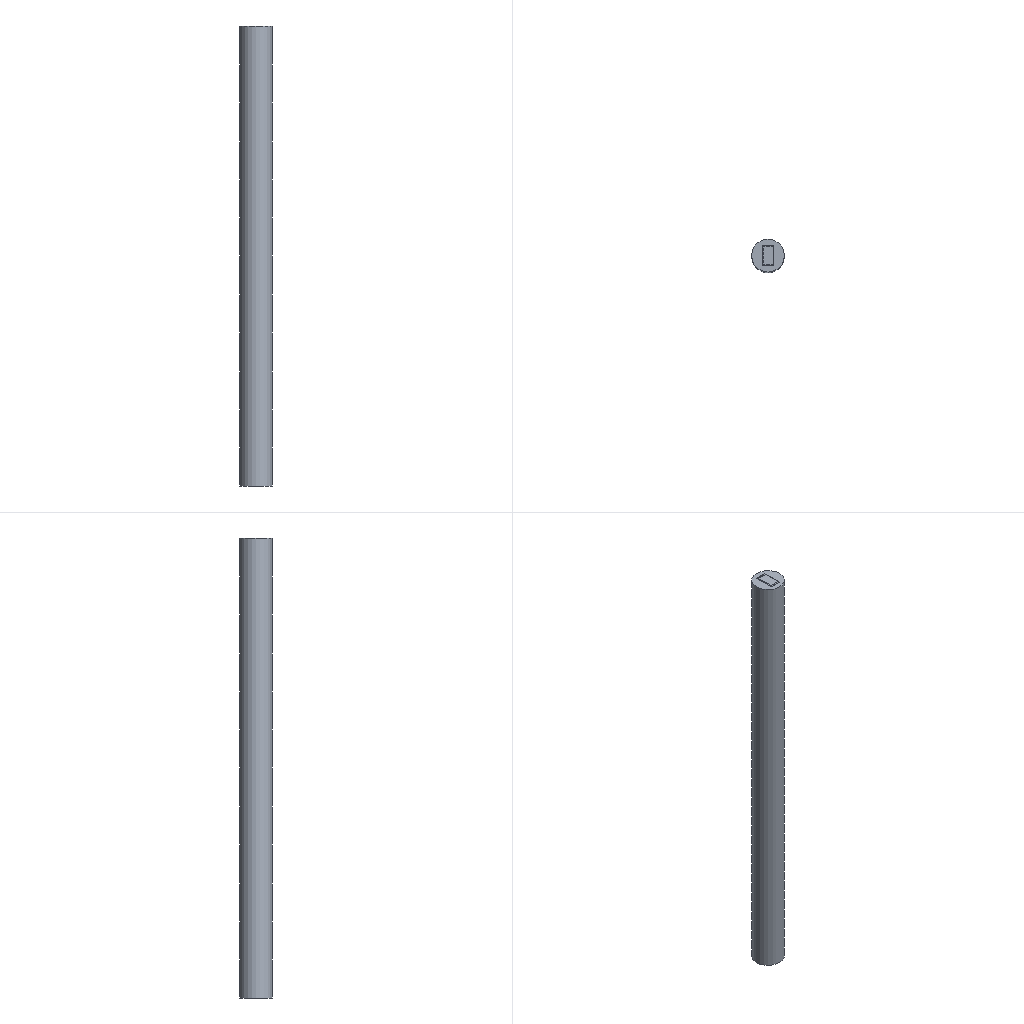Simulation study | abaqus
Set-up summary:
category,name,step,type,value,unit,region
solver,abaqus,,Abaqus/CAE 2024
units,mm-N-s-tonne (MPa),,inferred,E=206000 density=7.85e-09
analysis,Step-1,,dynamic explicit,nlgeom=True; time_period=0.02
mesh,nodes,,,88958
mesh,elements,,,66642
element_type,C3D8R,,,63378
element_type,S4R,,,2688
element_type,R3D4,,,384
element_type,T3D2,,,175
element_type,R3D3,,,16
element_type,MASS,,,1
material,CAOGANG,,E,206000
material,CAOGANG,,nu,0.3
material,CAOGANG,,density,7.85e-09
material,CAOGANG,,yield,235.322
material,CAOGANG,,behaviors,plastic; damage initiation; damage evolution
material,GFRP,,E,126000
material,GFRP,,nu,0.3
material,GFRP,,density,2e-09
material,GFRP,,behaviors,damage initiation; elastic engineering constants
material,HUNNINGTU,,E,36000
material,HUNNINGTU,,nu,0.25
material,HUNNINGTU,,density,2.5e-09
material,HUNNINGTU,,behaviors,plastic; concrete damaged plasticity; concrete compression hardening; concrete tension stiffening
material,gangjiaoxian,,E,195000
material,gangjiaoxian,,nu,0.3
material,gangjiaoxian,,density,7.85e-09
material,gangjiaoxian,,cte,1.2e-05
material,gangjiaoxian,,behaviors,expansion
section,CAOGANG,,solid section,,,_PickedSet15
section,,,shell section,0.1,,GFRP-1
section,HUNNINGTU,,solid section,,,_PickedSet3
section,HUNNINGTU,,solid section,,,_PickedSet2
section,gangjiaoxian,,solid section,,,_PickedSet2
load,Predefined,initial,initial condition temperature
load,qiu150,initial,initial condition velocity
load,Predefined,Step-1,temperature,-325,,Set-16
bc,gudingduan,initial,encastre,[dofs=ENCASTRE],,_PickedSet51
bc,qiu150,initial,fixed,"[dofs=rx,ry,rz,x,z n=5]",,_PickedSet89
bc,shuxiang,initial,fixed,"[dofs=rx,ry,rz,x,z n=5]",,_PickedSet52
contact,tu1-tu2,initial,tie,,,_PickedSurf47 / _PickedSurf46
contact,caonei-tu2,Step-1,contact pair,interaction=caonei-tu2; friction=0.6; behavior=hard,,_PickedSurf44 / _PickedSurf45
contact,caowai-tu1,Step-1,contact pair,interaction=caowai-tu1; friction=0.6; behavior=hard,,_PickedSurf42 / _PickedSurf43
contact,gfrp-hunningtu1,Step-1,contact pair,interaction=gfrp-hunningtu1; friction=0.6; behavior=hard,,_PickedSurf40 / _PickedSurf41
contact,qiu150-gfrp,Step-1,contact pair,interaction=qiu150-gfrp; friction=0; behavior=hard,,_PickedSurf67 / _PickedSurf68
constraint,embedded element,,,1
constraint,coupling,,,2
constraint,rigid body,,,1
Abaqus input file, long lists of numbers shortened:
*Heading
** Job name: deck Model name: CFFT-SP3-150-135-Copy
** Generated by: Abaqus/CAE 2024
*Preprint, echo=NO, model=NO, history=NO, contact=NO
**
** PARTS
**
*Part, name=CAOGANG
*Node
      1,          65.,          92.,           0.
      2,          65.,          92.,        1400.
** (22462 more lines like these left out)
*Element, type=C3D8R
   1,     8,  1091,  7807,  1453,     1,    21,  3619,   742
   2,  1091,  1090,  7808,  7807,    21,    22,  3620,  3619
** (10848 more lines like these left out)
*Nset, nset=Set-1, generate
     1,  22464,      1
*Elset, elset=Set-1, generate
     1,  10850,      1
*Nset, nset=_PickedSet15, internal, generate
     1,  22464,      1
*Elset, elset=_PickedSet15, internal, generate
     1,  10850,      1
** Section: CAOGANG
*Solid Section, elset=_PickedSet15, material=CAOGANG
,
*End Part
**
*Part, name=GFRP
*Node
      1,         -50.,           0.,        1400.
      2,         -50.,           0.,        1250.
** (2710 more lines like these left out)
*Element, type=S4R
 1,    1,   81, 1065,  108
 2,   81,   82, 1066, 1065
** (2686 more lines like these left out)
*Nset, nset=_PickedSet6, internal
    1,    4,   22,   25,   43,   46,   62,   65,  106,  107,  108,  345,  346,  347,  582,  799
  993, 1001, 1002, 1003, 1009, 1016, 1017, 1018
*Elset, elset=_PickedSet6, internal
    1,   13,   25,   37,  449,  461,  473,  485,  897,  909, 1121, 1133, 1356, 1368, 1428, 1440
 1452, 1464, 1500, 1512, 1572, 1584, 1596, 1608
*Elset, elset=__PickedSurf5_SPOS, internal, generate
    1,  2688,     1
*Surface, type=ELEMENT, name=_PickedSurf5, internal
__PickedSurf5_SPOS, SPOS
*Distribution, name=Ori-1-DiscOrient, location=ELEMENT, Table=Ori-1-DiscOrient_Table
** Description: Distribution generated from Discrete Orientation
,           1.,           0.,           0.,           0.,           1.,           0.
1, -0.1326, 0.9912,           0.,           0.,           0.,          -1.
2, -0.1326, 0.9912,           0.,           0.,           0.,          -1.
3, -0.1326, 0.9912,           0.,           0.,           0.,          -1.
4, -0.1326, 0.9912,           0.,           0.,           0.,          -1.
5, -0.1326, 0.9912,           0.,           0.,           0.,          -1.
6, -0.1326, 0.9912,           0.,           0.,           0.,          -1.
7, -0.1326, 0.9912,           0.,           0.,           0.,          -1.
8, -0.1326, 0.9912,           0.,           0.,           0.,          -1.
9, -0.1326, 0.9912,           0.,           0.,           0.,          -1.
10, -0.1326, 0.9912,           0.,           0.,           0.,          -1.
11, -0.1326, 0.9912,           0.,           0.,           0.,          -1.
12, -0.1326, 0.9912,           0.,           0.,           0.,          -1.
13, -0.3884, 0.9215,           0.,           0.,           0.,          -1.
14, -0.3884, 0.9215,           0.,           0.,           0.,          -1.
15, -0.3884, 0.9215,           0.,           0.,           0.,          -1.
16, -0.3884, 0.9215,           0.,           0.,           0.,          -1.
17, -0.3884, 0.9215,           0.,           0.,           0.,          -1.
18, -0.3884, 0.9215,           0.,           0.,           0.,          -1.
19, -0.3884, 0.9215,           0.,           0.,           0.,          -1.
20, -0.3884, 0.9215,           0.,           0.,           0.,          -1.
21, -0.3884, 0.9215,           0.,           0.,           0.,          -1.
22, -0.3884, 0.9215,           0.,           0.,           0.,          -1.
23, -0.3884, 0.9215,           0.,           0.,           0.,          -1.
24, -0.3884, 0.9215,           0.,           0.,           0.,          -1.
25, -0.6169, 0.787,           0.,           0.,           0.,          -1.
26, -0.6169, 0.787,           0.,           0.,           0.,          -1.
27, -0.6169, 0.787,           0.,           0.,           0.,          -1.
28, -0.6169, 0.787,           0.,           0.,           0.,          -1.
29, -0.6169, 0.787,           0.,           0.,           0.,          -1.
30, -0.6169, 0.787,           0.,           0.,           0.,          -1.
31, -0.6169, 0.787,           0.,           0.,           0.,          -1.
32, -0.6169, 0.787,           0.,           0.,           0.,          -1.
33, -0.6169, 0.787,           0.,           0.,           0.,          -1.
34, -0.6169, 0.787,           0.,           0.,           0.,          -1.
35, -0.6169, 0.787,           0.,           0.,           0.,          -1.
36, -0.6169, 0.787,           0.,           0.,           0.,          -1.
37, -0.8021, 0.5972,           0.,           0.,           0.,          -1.
38, -0.8021, 0.5972,           0.,           0.,           0.,          -1.
39, -0.8021, 0.5972,           0.,           0.,           0.,          -1.
** (2649 more lines like these left out)
*Orientation, name=Ori-1, system=RECTANGULAR
Ori-1-DiscOrient
3, 0.
** Region: (GFRP-1: Generated From Layup)
*Elset, elset=GFRP-1, generate
    1,  2688,     1
** Section: GFRP-1
*Shell Section, elset=GFRP-1, composite, orientation=Ori-1, offset=SNEG, layup=GFRP
0.1, 3, GFRP, 80., 层-1
0.1, 3, GFRP, -80., 层-2
0.1, 3, GFRP, 80., 层-3
*End Part
**
*Part, name=HUNNINGTU1
*Node
      1,        -17.5,           0.,        1400.
      2,         -50.,           0.,        1400.
** (18982 more lines like these left out)
*Element, type=C3D8R
   1,   286,  2649, 10105,  1983,     1,    33,  1953,    48
   2,  2649,  2650, 10106, 10105,    33,    34,  1954,  1953
** (16126 more lines like these left out)
*Nset, nset=_PickedSet3, internal, generate
     1,  18984,      1
*Elset, elset=_PickedSet3, internal, generate
     1,  16128,      1
** Section: HUNNINGTU
*Solid Section, elset=_PickedSet3, material=HUNNINGTU
,
*End Part
**
*Part, name=HUNNINGTU2
*Node
      1,         100.,          97.,        1400.
      2,       96.125,          97.,        1400.
** (44224 more lines like these left out)
*Element, type=C3D8R
    1,  3160,  3161,  3170,  3169,     1,     2,    11,    10
    2,  3161,  3162,  3171,  3170,     2,     3,    12,    11
** (36398 more lines like these left out)
*Nset, nset=_PickedSet2, internal, generate
     1,  44226,      1
*Elset, elset=_PickedSet2, internal, generate
     1,  36400,      1
** Section: HUNNINGTU
*Solid Section, elset=_PickedSet2, material=HUNNINGTU
,
*End Part
**
*Part, name=QIU100
*Node
      1,          50.,           0.,           0.
      2,           0.,           0.,          50.
** (392 more lines like these left out)
*Element, type=R3D3
1, 108, 107, 122
2, 126, 113, 109
** (14 more lines like these left out)
*Element, type=R3D4
 3,   7,  93,  27,   1
 4, 114,  93,  92, 115
** (382 more lines like these left out)
*End Part
**
*Part, name=gangjiaoxian
*Node
      1,       -1075.,           0.,           0.
      2,       -1067.,           0.,           0.
** (174 more lines like these left out)
*Element, type=T3D2
  1,   1,   2
  2,   2,   3
** (173 more lines like these left out)
*Nset, nset=_PickedSet2, internal, generate
   1,  176,    1
*Elset, elset=_PickedSet2, internal, generate
   1,  175,    1
** Section: gangjiaoxian
*Solid Section, elset=_PickedSet2, material=gangjiaoxian
140.,
*End Part
**
**
** ASSEMBLY
**
*Assembly, name=Assembly
**
*Instance, name=GFRP-1, part=GFRP
*End Instance
**
*Instance, name=HUNNINGTU1-1, part=HUNNINGTU1
*End Instance
**
*Instance, name=CAOGANG-1, part=CAOGANG
       -82.5,       -118.5,           0.
*End Instance
**
*Instance, name=HUNNINGTU2-1, part=HUNNINGTU2
       -82.5,       -123.5,           0.
*End Instance
**
*Instance, name=QIU100-1, part=QIU100
          0.,         176.,        1250.
*End Instance
**
*Instance, name=gangjiaoxian-1, part=gangjiaoxian
7.95145259115256e-14,           0., 325.
7.95145259115256e-14,           0., 325., 7.95145259115256e-14, 1., 325., 90.
*End Instance
**
*Node
      1,           0.,           0.,           0.
*Node
      2,           0.,         226.,        1250.
*Nset, nset=Set-16, instance=gangjiaoxian-1, generate
   1,  176,    1
*Elset, elset=Set-16, instance=gangjiaoxian-1, generate
   1,  175,    1
*Nset, nset=jiasudu, instance=HUNNINGTU1-1
 1373, 1405, 1433
*Nset, nset=weiyi, instance=HUNNINGTU1-1
   21, 1369, 1393, 1417, 1441
*Nset, nset=yingbian, instance=HUNNINGTU1-1
   21, 1349, 1365, 1377, 1401, 1413, 1437
*Nset, nset=_PickedSet51, internal, instance=HUNNINGTU1-1
    5,    6,    7,    8,   13,   14,   15,   16,   21,   22,   23,   24,   27,   28,   31,   32
   49,   50,   51,   52,   53,   54,   55,   56,   57,   58,   59,   60,   61,   62,   63,   64
** (9 more lines like these left out)
*Nset, nset=_PickedSet51, internal, instance=CAOGANG-1
    1,    4,    7,    8,   11,   12,   14,   17,   18,   19,  731,  732,  733,  734,  735,  736
  737,  738,  739,  740,  741,  742, 1453, 1454, 1455, 1456, 1457, 1458, 1459, 1460, 1461, 1462
** (2 more lines like these left out)
*Nset, nset=_PickedSet51, internal, instance=HUNNINGTU2-1
  3151,  3152,  3153,  3154,  3155,  3156,  3157,  3158,  3159,  6310,  6311,  6312,  6313,  6314,  6315,  6316
  6317,  6318,  9469,  9470,  9471,  9472,  9473,  9474,  9475,  9476,  9477, 12628, 12629, 12630, 12631, 12632
** (6 more lines like these left out)
*Elset, elset=_PickedSet51, internal, instance=HUNNINGTU1-1
  2665,  2666,  2667,  2668,  2669,  2670,  2671,  2672,  2673,  2674,  2675,  2676,  2677,  2678,  2679,  2680
  2681,  2682,  2683,  2684,  2685,  2686,  2687,  2688,  5353,  5354,  5355,  5356,  5357,  5358,  5359,  5360
** (7 more lines like these left out)
*Elset, elset=_PickedSet51, internal, instance=CAOGANG-1
     1,   351,   701,  1051,  1401,  1751,  2101,  2451,  2801,  3151,  3501,  3851,  4201,  4900,  5250,  5600
  5950,  6300,  6650,  7000,  7350,  7700,  8050,  8400,  8750,  9100,  9450,  9800, 10150, 10500, 10850
*Elset, elset=_PickedSet51, internal, instance=HUNNINGTU2-1
  2793,  2794,  2795,  2796,  2797,  2798,  2799,  2800,  5593,  5594,  5595,  5596,  5597,  5598,  5599,  5600
  8393,  8394,  8395,  8396,  8397,  8398,  8399,  8400, 11193, 11194, 11195, 11196, 11197, 11198, 11199, 11200
** (5 more lines like these left out)
*Nset, nset=_PickedSet52, internal, instance=HUNNINGTU1-1
   2,   5,  10,  13, 398, 399, 400, 401, 402, 403, 404, 405, 406, 407, 408, 409
 410, 411, 412, 413, 414, 415, 416, 417, 418, 419, 420, 421, 422, 423, 424, 425
** (13 more lines like these left out)
*Elset, elset=_PickedSet52, internal, instance=HUNNINGTU1-1
     6,    30,    54,    78,   102,   126,   150,   174,   198,   222,   246,   270,   294,   318,   342,   366
   390,   414,   438,   462,   486,   510,   534,   558,   582,   606,   630,   654,   678,   702,   726,   750
** (26 more lines like these left out)
*Nset, nset=_PickedSet62, internal
 1,
*Nset, nset=_PickedSet63, internal, instance=HUNNINGTU1-1
    5,    6,   13,   14,   21,   22,   28,   32,   54,   55,   56,  530,  531,  532, 1002, 1466
 1708, 1709, 1710, 1942, 1943, 1944, 1947, 1952
*Elset, elset=_PickedSet63, internal, instance=HUNNINGTU1-1
  2670,  2676,  2682,  2688,  5358,  5364,  5370,  5376,  6714,  6720,  8053,  8059, 10729, 10735, 10741, 10747
 13417, 13423, 13429, 13435, 14778, 14784, 16117, 16123
*Nset, nset=_PickedSet64, internal
 1,
*Nset, nset=_PickedSet71, internal, instance=QIU100-1, generate
   1,  394,    1
*Elset, elset=_PickedSet71, internal, instance=QIU100-1, generate
   1,  400,    1
*Nset, nset=_PickedSet84, internal, instance=gangjiaoxian-1, generate
   1,  176,    1
*Elset, elset=_PickedSet84, internal, instance=gangjiaoxian-1, generate
   1,  175,    1
*Nset, nset=_PickedSet87, internal
 2,
*Nset, nset=_PickedSet88, internal
 2,
*Nset, nset=_PickedSet89, internal
 2,
*Elset, elset=__PickedSurf40_SNEG, internal, instance=GFRP-1, generate
    1,  2688,     1
*Surface, type=ELEMENT, name=_PickedSurf40, internal
__PickedSurf40_SNEG, SNEG
*Elset, elset=__PickedSurf41_S4, internal, instance=HUNNINGTU1-1
     6,    12,    18,    24,    30,    36,    42,    48,    54,    60,    66,    72,    78,    84,    90,    96
   102,   108,   114,   120,   126,   132,   138,   144,   150,   156,   162,   168,   174,   180,   186,   192
** (82 more lines like these left out)
*Elset, elset=__PickedSurf41_S6, internal, instance=HUNNINGTU1-1
  6721,  6727,  6733,  6739,  6745,  6751,  6757,  6763,  6769,  6775,  6781,  6787,  6793,  6799,  6805,  6811
  6817,  6823,  6829,  6835,  6841,  6847,  6853,  6859,  6865,  6871,  6877,  6883,  6889,  6895,  6901,  6907
** (82 more lines like these left out)
*Surface, type=ELEMENT, name=_PickedSurf41, internal
__PickedSurf41_S4, S4
__PickedSurf41_S6, S6
*Elset, elset=__PickedSurf42_S2, internal, instance=CAOGANG-1
    1,    2,    3,    4,    5,    6,    7,    8,    9,   10,   11,   12,   13,   14,   15,   16
   17,   18,   19,   20,   21,   22,   23,   24,   25,   26,   27,   28,   29,   30,   31,   32
** (327 more lines like these left out)
*Elset, elset=__PickedSurf42_S1, internal, instance=CAOGANG-1
  7351,  7352,  7353,  7354,  7355,  7356,  7357,  7358,  7359,  7360,  7361,  7362,  7363,  7364,  7365,  7366
  7367,  7368,  7369,  7370,  7371,  7372,  7373,  7374,  7375,  7376,  7377,  7378,  7379,  7380,  7381,  7382
** (42 more lines like these left out)
*Elset, elset=__PickedSurf42_S6, internal, instance=CAOGANG-1, generate
  7701,  10850,      1
*Elset, elset=__PickedSurf42_S4, internal, instance=CAOGANG-1, generate
 4551,  7700,     1
*Surface, type=ELEMENT, name=_PickedSurf42, internal
__PickedSurf42_S2, S2
__PickedSurf42_S1, S1
__PickedSurf42_S6, S6
__PickedSurf42_S4, S4
*Elset, elset=__PickedSurf43_S4, internal, instance=HUNNINGTU1-1
  6726,  6732,  6738,  6744,  6750,  6756,  6762,  6768,  6774,  6780,  6786,  6792,  6798,  6804,  6810,  6816
  6822,  6828,  6834,  6840,  6846,  6852,  6858,  6864,  6870,  6876,  6882,  6888,  6894,  6900,  6906,  6912
** (82 more lines like these left out)
*Elset, elset=__PickedSurf43_S6, internal, instance=HUNNINGTU1-1
     1,     7,    13,    19,    25,    31,    37,    43,    49,    55,    61,    67,    73,    79,    85,    91
    97,   103,   109,   115,   121,   127,   133,   139,   145,   151,   157,   163,   169,   175,   181,   187
** (82 more lines like these left out)
*Surface, type=ELEMENT, name=_PickedSurf43, internal
__PickedSurf43_S4, S4
__PickedSurf43_S6, S6
*Elset, elset=__PickedSurf44_S4, internal, instance=CAOGANG-1, generate
  7701,  10500,      1
*Elset, elset=__PickedSurf44_S1, internal, instance=CAOGANG-1, generate
    1,  4550,     1
*Elset, elset=__PickedSurf44_S6, internal, instance=CAOGANG-1, generate
 4551,  7350,     1
*Surface, type=ELEMENT, name=_PickedSurf44, internal
__PickedSurf44_S4, S4
__PickedSurf44_S1, S1
__PickedSurf44_S6, S6
*Elset, elset=__PickedSurf45_S1, internal, instance=HUNNINGTU2-1, generate
 33601,  36400,      1
*Elset, elset=__PickedSurf45_S2, internal, instance=HUNNINGTU2-1, generate
    1,  2800,     1
*Elset, elset=__PickedSurf45_S4, internal, instance=HUNNINGTU2-1, generate
     8,  36400,      8
*Surface, type=ELEMENT, name=_PickedSurf45, internal
__PickedSurf45_S1, S1
__PickedSurf45_S2, S2
__PickedSurf45_S4, S4
*Elset, elset=__PickedSurf46_S4, internal, instance=HUNNINGTU1-1, generate
  8070,  10752,      6
*Elset, elset=__PickedSurf46_S6, internal, instance=HUNNINGTU1-1, generate
 2689,  5371,     6
*Surface, type=ELEMENT, name=_PickedSurf46, internal
__PickedSurf46_S4, S4
__PickedSurf46_S6, S6
*Elset, elset=__PickedSurf47_S6, internal, instance=HUNNINGTU2-1, generate
     1,  36393,      8
*Surface, type=ELEMENT, name=_PickedSurf47, internal
__PickedSurf47_S6, S6
*Elset, elset=__PickedSurf61_S1, internal, instance=HUNNINGTU1-1
  2665,  2666,  2667,  2668,  2669,  2670,  2671,  2672,  2673,  2674,  2675,  2676,  2677,  2678,  2679,  2680
  2681,  2682,  2683,  2684,  2685,  2686,  2687,  2688,  5353,  5354,  5355,  5356,  5357,  5358,  5359,  5360
** (7 more lines like these left out)
*Elset, elset=__PickedSurf61_S5, internal, instance=CAOGANG-1, generate
  4900,  10850,    350
*Elset, elset=__PickedSurf61_S5, internal, instance=HUNNINGTU2-1
  2793,  2794,  2795,  2796,  2797,  2798,  2799,  2800,  5593,  5594,  5595,  5596,  5597,  5598,  5599,  5600
  8393,  8394,  8395,  8396,  8397,  8398,  8399,  8400, 11193, 11194, 11195, 11196, 11197, 11198, 11199, 11200
** (5 more lines like these left out)
*Elset, elset=__PickedSurf61_S6, internal, instance=CAOGANG-1, generate
    1,  4201,   350
*Surface, type=ELEMENT, name=_PickedSurf61, internal
__PickedSurf61_S1, S1
__PickedSurf61_S5, S5
__PickedSurf61_S6, S6
*Elset, elset=__PickedSurf67_SPOS, internal, instance=QIU100-1
   1,   2,   3,   4,   5,   6,   7,   8,   9,  10,  11,  12,  13,  14,  15,  16
  17,  18,  19,  20,  21,  22,  23,  24,  25,  26,  27,  28,  29,  30,  31,  32
** (11 more lines like these left out)
*Surface, type=ELEMENT, name=_PickedSurf67, internal
__PickedSurf67_SPOS, SPOS
*Elset, elset=__PickedSurf68_SPOS, internal, instance=GFRP-1
    1,    2,    3,    4,    5,    6,    7,    8,    9,   10,   11,   12,   13,   14,   15,   16
   17,   18,   19,   20,   21,   22,   23,   24,   25,   26,   27,   28,   29,   30,   31,   32
** (34 more lines like these left out)
*Surface, type=ELEMENT, name=_PickedSurf68, internal
__PickedSurf68_SPOS, SPOS
*Surface, type=NODE, name=_PickedSet63_CNS_, internal
_PickedSet63, 1.
** Constraint: gangjioaxian-hun2
*Embedded Element
_PickedSet84
** Constraint: guding-gfrp
*Coupling, constraint name=guding-gfrp, ref node=_PickedSet64, surface=_PickedSet63_CNS_
*Kinematic
** Constraint: gudingduan
*Coupling, constraint name=gudingduan, ref node=_PickedSet62, surface=_PickedSurf61
*Kinematic
** Constraint: qiu150
*Rigid Body, ref node=_PickedSet87, elset=_PickedSet71
** Constraint: tu1-tu2
*Tie, name=tu1-tu2, adjust=yes
_PickedSurf47, _PickedSurf46
*Element, type=MASS, elset=_PickedSet86_qiu150_
1, 2
*Mass, elset=_PickedSet86_qiu150_
0.0139,
*End Assembly
*Distribution Table, name=Ori-1-DiscOrient_Table
coord3D, coord3D
*Amplitude, name=Amp-1
             0.,              0.,            0.01,              1.
**
** MATERIALS
**
*Material, name=CAOGANG
*Damage Initiation, criterion=DUCTILE
 0.44,  1.29, 4.375
*Damage Evolution, type=DISPLACEMENT
 8.8,
*Density
 7.85e-09,
*Elastic
206000., 0.3
*Plastic
 235.322,         0.
 235.611, 0.001454
 235.901, 0.002681
  236.19, 0.003906
  236.48, 0.005129
 236.769, 0.006352
 237.059, 0.007572
 237.348, 0.008791
 237.638,  0.01001
 237.927,  0.01123
 238.217,  0.01244
 255.579,  0.02444
 273.288,  0.03629
 291.345,  0.048
  309.75,  0.05956
 328.501,  0.071
 347.601,  0.0823
 367.047,  0.09347
 386.841,   0.1045
 406.983,   0.1154
 427.472,   0.1262
 436.737,   0.1476
 446.002,   0.1686
 455.267,   0.1891
 464.532,   0.2092
 473.797,   0.2289
 483.061,    0.2482
 492.326,   0.2672
 501.591,   0.2858
*Material, name=GFRP
*Damage Initiation, criterion=HASHIN
560.,240., 30.,100., 65., 20.
*Density
 2e-09,
*Elastic, type=ENGINEERING CONSTANTS
126000.,4600.,4600.,  0.3,  0.3, 0.28,2400.,2400.
1600.,
*Material, name=HUNNINGTU
*Density
 2.5e-09,
*Elastic
36000., 0.25
*Concrete Damaged Plasticity
36.,    0.1,   1.16, 0.6667,  1e-05
*Concrete Compression Hardening
  24.9,       0.
  35.3, 0.000728
 18.98,  0.00293
 10.96,  0.00485
 7.432,   0.0068
  5.61,   0.0085
  3.71,  0.01203
  3.15,   0.0141
  2.75,   0.0155
*Concrete Tension Stiffening
  2.801,        0.
  2.736,  3.51e-05
 1.27, 0.0001901
  0.776, 0.0003183
  0.573,  0.000436
  0.461, 0.0005512
  0.392,  0.000658
  0.277,  0.001004
  0.091,   0.00451
*Material, name=gangjiaoxian
*Density
 7.85e-09,
*Elastic
195000., 0.3
*Expansion
 1.2e-05,
**
** INTERACTION PROPERTIES
**
*Surface Interaction, name=caonei-tu2
*Friction
 0.6,
*Surface Behavior, pressure-overclosure=HARD
*Surface Interaction, name=caowai-tu1
*Friction
 0.6,
*Surface Behavior, pressure-overclosure=HARD
*Surface Interaction, name=gfrp-hunningtu1
*Friction
 0.6,
*Surface Behavior, pressure-overclosure=HARD
*Surface Interaction, name=qiu150-gfrp
*Friction
0.,
*Surface Behavior, pressure-overclosure=HARD
**
** BOUNDARY CONDITIONS
**
** Name: gudingduan Type: Symmetry/Antisymmetry/Encastre
*Boundary
_PickedSet51, ENCASTRE
** Name: qiu150 Type: Displacement/Rotation
*Boundary
_PickedSet89, 1, 1
_PickedSet89, 3, 3
_PickedSet89, 4, 4
_PickedSet89, 5, 5
_PickedSet89, 6, 6
** Name: shuxiang Type: Displacement/Rotation
*Boundary
_PickedSet52, 1, 1
_PickedSet52, 3, 3
_PickedSet52, 4, 4
_PickedSet52, 5, 5
_PickedSet52, 6, 6
**
** PREDEFINED FIELDS
**
** Name: Predefined Field-2   Type: Temperature
*Initial Conditions, type=TEMPERATURE
Set-16, 20.
** Name: qiu150   Type: Velocity
*Initial Conditions, type=VELOCITY
_PickedSet88, 2, -7000.
** ----------------------------------------------------------------
**
** STEP: Step-1
**
*Step, name=Step-1, nlgeom=YES
*Dynamic, Explicit
, 0.02
*Bulk Viscosity
0.06, 1.2
** Mass Scaling: Semi-Automatic
**               Whole Model
*Fixed Mass Scaling, factor=1000.
**
** PREDEFINED FIELDS
**
** Name: Predefined Field-2   Type: Temperature
*Temperature, amplitude=Amp-1
Set-16, -325.
**
** INTERACTIONS
**
** Interaction: caonei-tu2
*Contact Pair, interaction=caonei-tu2, mechanical constraint=KINEMATIC, cpset=caonei-tu2
_PickedSurf44, _PickedSurf45
** Interaction: caowai-tu1
*Contact Pair, interaction=caowai-tu1, mechanical constraint=KINEMATIC, cpset=caowai-tu1
_PickedSurf42, _PickedSurf43
** Interaction: gfrp-hunningtu1
*Contact Pair, interaction=gfrp-hunningtu1, mechanical constraint=KINEMATIC, cpset=gfrp-hunningtu1
_PickedSurf40, _PickedSurf41
** Interaction: qiu150-gfrp
*Contact Pair, interaction=qiu150-gfrp, mechanical constraint=KINEMATIC, cpset=qiu150-gfrp
_PickedSurf67, _PickedSurf68
**
** OUTPUT REQUESTS
**
*Restart, write, number interval=1, time marks=NO
**
** FIELD OUTPUT: F-Output-1
**
*Output, field
*Node Output
A, RF, U, V
*Element Output, directions=YES
EVF, LE, PE, PEEQ, PEEQVAVG, PEVAVG, S, STATUS, SVAVG
*Contact Output
CSTRESS,
**
** HISTORY OUTPUT: H-Output-1
**
*Output, history
*Energy Output
ALLIE, ALLKE
**
** HISTORY OUTPUT: H-Output-5
**
*Contact Output, cpset=qiu150-gfrp
CFN2,
**
** HISTORY OUTPUT: H-Output-2
**
*Node Output, nset=jiasudu
A2,
**
** HISTORY OUTPUT: H-Output-3
**
*Node Output, nset=weiyi
U2,
**
** HISTORY OUTPUT: H-Output-4
**
*End Step
Results summary:
result,odb.job_status,,,JOB_STATUS_COMPLETED_SUCCESSFULLY,"consistent, unstated (Abaqus has no unit system)"
result,steps[0].procedure,Step-1,,"*DYNAMIC, EXPLICIT","consistent, unstated (Abaqus has no unit system)"
result,steps[0].time_period,Step-1,,0.02,"consistent, unstated (Abaqus has no unit system)"
result,steps[0].n_frames,Step-1,,21,"consistent, unstated (Abaqus has no unit system)"
result,steps[0].last_frame.id,Step-1,,2404,"consistent, unstated (Abaqus has no unit system)"
result,steps[0].last_frame.value,Step-1,,0.02,"consistent, unstated (Abaqus has no unit system)"
result,steps[0].last_frame.description,Step-1,,Increment      2404: Step Time =   2.0000E-02,"consistent, unstated (Abaqus has no unit system)"
result,steps[0].completed,Step-1,,True,"consistent, unstated (Abaqus has no unit system)"
result,steps[0].max_U_magnitude,Step-1,,137.784,"consistent, unstated (Abaqus has no unit system)"
result,steps[0].max_S_mises,Step-1,,24697.6,"consistent, unstated (Abaqus has no unit system)"
result,steps[0].RF_sum[1],Step-1,,93258.5,"consistent, unstated (Abaqus has no unit system)"
result,steps[0].RF_sum[2],Step-1,,-289.157,"consistent, unstated (Abaqus has no unit system)"
result,steps[0].RF_sum[3],Step-1,,85848.2,"consistent, unstated (Abaqus has no unit system)"
result,steps[0].diagnostic.n_increments,Step-1,,21,"consistent, unstated (Abaqus has no unit system)"